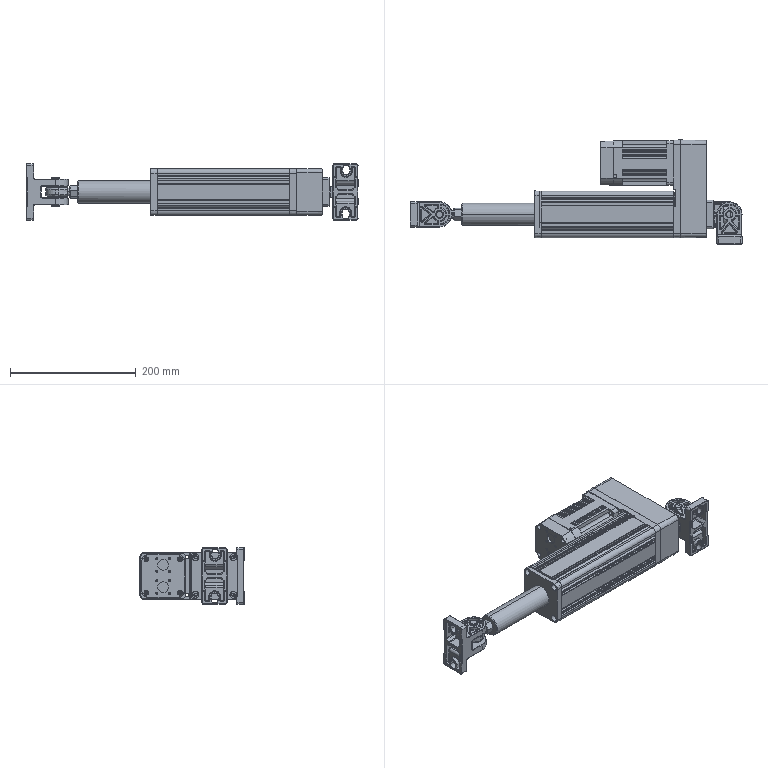Part | SolidWorks | 15 solids | 2607 faces | box 527.291 x 165.21 x 90 mm | volume 1479501 mm3 | cylinder 1007 | plane 682 | spline 578 | cone 300 | torus 40 | commonest cylinder face diameters 1.2 x184 2 x180 3 x154 0.6 x56 4 x40 5 x28